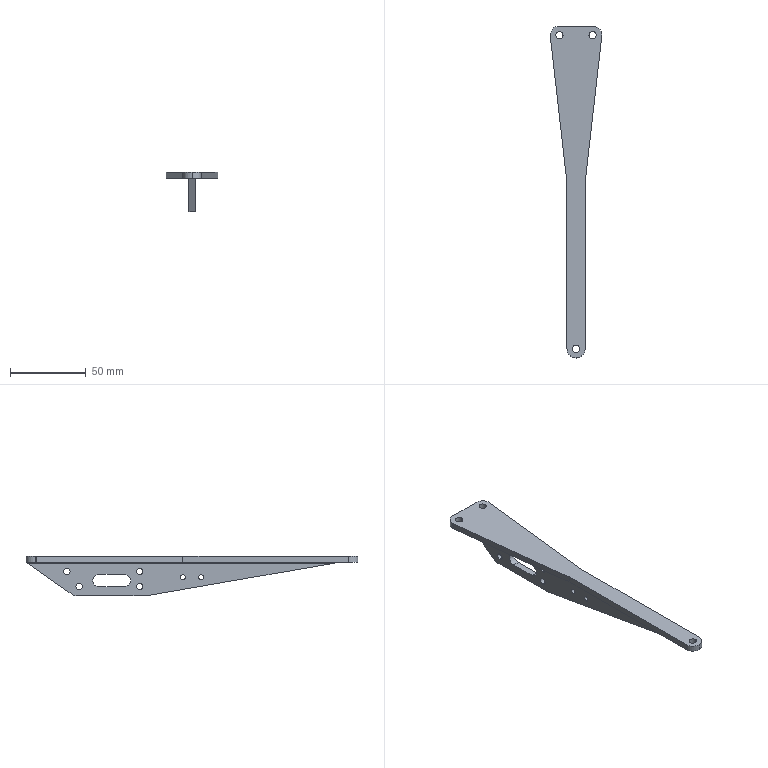Part | SolidWorks | features BaseBody 1 | 1 solid | 44 faces | box 34 x 219 x 26 mm | volume 25249 mm3 | cylinder 29 | plane 15 | commonest cylinder face diameters 4.2 x8 4.9 x6 12 x5 3.2 x4 2 x2 8 x2
STEP:
#1=CARTESIAN_POINT('',(2.,103.5,-12.2));
#2=VERTEX_POINT('',#1);
#3=CARTESIAN_POINT('',(2.,103.5,-15.4));
#4=VERTEX_POINT('',#3);
#5=CARTESIAN_POINT('',(2.,103.5,-13.8));
#6=DIRECTION('',(1.,0.,0.));
#7=DIRECTION('',(0.,0.,1.));
#8=AXIS2_PLACEMENT_3D('',#5,#6,#7);
#9=CIRCLE('',#8,1.6);
#10=EDGE_CURVE('',#2,#4,#9,.T.);
#11=ORIENTED_EDGE('',*,*,#10,.T.);
#12=CARTESIAN_POINT('',(-2.,103.5,-15.4));
#13=VERTEX_POINT('',#12);
#14=CARTESIAN_POINT('',(2.,103.5,-15.4));
#15=DIRECTION('',(-1.,0.,0.));
#16=VECTOR('',#15,1000.);
#17=LINE('',#14,#16);
#18=EDGE_CURVE('',#4,#13,#17,.T.);
#19=ORIENTED_EDGE('',*,*,#18,.T.);
#20=CARTESIAN_POINT('',(-2.,103.5,-12.2));
#21=VERTEX_POINT('',#20);
#22=CARTESIAN_POINT('',(-2.,103.5,-13.8));
#23=DIRECTION('',(-1.,0.,0.));
#24=DIRECTION('',(0.,0.,1.));
#25=AXIS2_PLACEMENT_3D('',#22,#23,#24);
#26=CIRCLE('',#25,1.6);
#27=EDGE_CURVE('',#13,#21,#26,.T.);
#28=ORIENTED_EDGE('',*,*,#27,.T.);
#29=CARTESIAN_POINT('',(2.,103.5,-12.2));
#30=DIRECTION('',(-1.,0.,0.));
#31=VECTOR('',#30,1000.);
#32=LINE('',#29,#31);
#33=EDGE_CURVE('',#2,#21,#32,.T.);
#34=ORIENTED_EDGE('',*,*,#33,.F.);
#35=EDGE_LOOP('',(#11,#19,#28,#34));
#36=FACE_OUTER_BOUND('',#35,.T.);
#37=CARTESIAN_POINT('',(2.,103.5,-13.8));
#38=DIRECTION('',(-1.,0.,0.));
#39=DIRECTION('',(0.,0.,1.));
#40=AXIS2_PLACEMENT_3D('',#37,#38,#39);
#41=CYLINDRICAL_SURFACE('',#40,1.6);
#42=ADVANCED_FACE('',(#36),#41,.F.);
#43=CARTESIAN_POINT('',(2.,184.,-17.9));
#44=VERTEX_POINT('',#43);
#45=CARTESIAN_POINT('',(2.,184.,-22.1));
#46=VERTEX_POINT('',#45);
#47=CARTESIAN_POINT('',(2.,184.,-20.));
#48=DIRECTION('',(1.,0.,0.));
#49=DIRECTION('',(0.,0.,1.));
#50=AXIS2_PLACEMENT_3D('',#47,#48,#49);
#51=CIRCLE('',#50,2.1);
#52=EDGE_CURVE('',#44,#46,#51,.T.);
#53=ORIENTED_EDGE('',*,*,#52,.T.);
#54=CARTESIAN_POINT('',(-2.,184.,-22.1));
#55=VERTEX_POINT('',#54);
#56=CARTESIAN_POINT('',(2.,184.,-22.1));
#57=DIRECTION('',(-1.,0.,0.));
#58=VECTOR('',#57,1000.);
#59=LINE('',#56,#58);
#60=EDGE_CURVE('',#46,#55,#59,.T.);
#61=ORIENTED_EDGE('',*,*,#60,.T.);
#62=CARTESIAN_POINT('',(-2.,184.,-17.9));
#63=VERTEX_POINT('',#62);
#64=CARTESIAN_POINT('',(-2.,184.,-20.));
#65=DIRECTION('',(-1.,0.,0.));
#66=DIRECTION('',(0.,0.,1.));
#67=AXIS2_PLACEMENT_3D('',#64,#65,#66);
#68=CIRCLE('',#67,2.1);
#69=EDGE_CURVE('',#55,#63,#68,.T.);
#70=ORIENTED_EDGE('',*,*,#69,.T.);
#71=CARTESIAN_POINT('',(2.,184.,-17.9));
#72=DIRECTION('',(-1.,0.,0.));
#73=VECTOR('',#72,1000.);
#74=LINE('',#71,#73);
#75=EDGE_CURVE('',#44,#63,#74,.T.);
#76=ORIENTED_EDGE('',*,*,#75,.F.);
#77=EDGE_LOOP('',(#53,#61,#70,#76));
#78=FACE_OUTER_BOUND('',#77,.T.);
#79=CARTESIAN_POINT('',(2.,184.,-20.));
#80=DIRECTION('',(-1.,0.,0.));
#81=DIRECTION('',(0.,0.,1.));
#82=AXIS2_PLACEMENT_3D('',#79,#80,#81);
#83=CYLINDRICAL_SURFACE('',#82,2.1);
#84=ADVANCED_FACE('',(#78),#83,.F.);
#85=CARTESIAN_POINT('',(2.,192.,-7.9));
#86=VERTEX_POINT('',#85);
#87=CARTESIAN_POINT('',(2.,192.,-12.1));
#88=VERTEX_POINT('',#87);
#89=CARTESIAN_POINT('',(2.,192.,-10.));
#90=DIRECTION('',(1.,0.,0.));
#91=DIRECTION('',(0.,0.,1.));
#92=AXIS2_PLACEMENT_3D('',#89,#90,#91);
#93=CIRCLE('',#92,2.1);
#94=EDGE_CURVE('',#86,#88,#93,.T.);
#95=ORIENTED_EDGE('',*,*,#94,.T.);
#96=CARTESIAN_POINT('',(-2.,192.,-12.1));
#97=VERTEX_POINT('',#96);
#98=CARTESIAN_POINT('',(2.,192.,-12.1));
#99=DIRECTION('',(-1.,0.,0.));
#100=VECTOR('',#99,1000.);
#101=LINE('',#98,#100);
#102=EDGE_CURVE('',#88,#97,#101,.T.);
#103=ORIENTED_EDGE('',*,*,#102,.T.);
#104=CARTESIAN_POINT('',(-2.,192.,-7.9));
#105=VERTEX_POINT('',#104);
#106=CARTESIAN_POINT('',(-2.,192.,-10.));
#107=DIRECTION('',(-1.,0.,0.));
#108=DIRECTION('',(0.,0.,1.));
#109=AXIS2_PLACEMENT_3D('',#106,#107,#108);
#110=CIRCLE('',#109,2.1);
#111=EDGE_CURVE('',#97,#105,#110,.T.);
#112=ORIENTED_EDGE('',*,*,#111,.T.);
#113=CARTESIAN_POINT('',(2.,192.,-7.9));
#114=DIRECTION('',(-1.,0.,0.));
#115=VECTOR('',#114,1000.);
#116=LINE('',#113,#115);
#117=EDGE_CURVE('',#86,#105,#116,.T.);
#118=ORIENTED_EDGE('',*,*,#117,.F.);
#119=EDGE_LOOP('',(#95,#103,#112,#118));
#120=FACE_OUTER_BOUND('',#119,.T.);
#121=CARTESIAN_POINT('',(2.,192.,-10.));
#122=DIRECTION('',(-1.,0.,0.));
#123=DIRECTION('',(0.,0.,1.));
#124=AXIS2_PLACEMENT_3D('',#121,#122,#123);
#125=CYLINDRICAL_SURFACE('',#124,2.1);
#126=ADVANCED_FACE('',(#120),#125,.F.);
#127=CARTESIAN_POINT('',(2.,144.,-17.9));
#128=VERTEX_POINT('',#127);
#129=CARTESIAN_POINT('',(2.,144.,-22.1));
#130=VERTEX_POINT('',#129);
#131=CARTESIAN_POINT('',(2.,144.,-20.));
#132=DIRECTION('',(1.,0.,0.));
#133=DIRECTION('',(0.,0.,1.));
#134=AXIS2_PLACEMENT_3D('',#131,#132,#133);
#135=CIRCLE('',#134,2.1);
#136=EDGE_CURVE('',#128,#130,#135,.T.);
#137=ORIENTED_EDGE('',*,*,#136,.T.);
#138=CARTESIAN_POINT('',(-2.,144.,-22.1));
#139=VERTEX_POINT('',#138);
#140=CARTESIAN_POINT('',(2.,144.,-22.1));
#141=DIRECTION('',(-1.,0.,0.));
#142=VECTOR('',#141,1000.);
#143=LINE('',#140,#142);
#144=EDGE_CURVE('',#130,#139,#143,.T.);
#145=ORIENTED_EDGE('',*,*,#144,.T.);
#146=CARTESIAN_POINT('',(-2.,144.,-17.9));
#147=VERTEX_POINT('',#146);
#148=CARTESIAN_POINT('',(-2.,144.,-20.));
#149=DIRECTION('',(-1.,0.,0.));
#150=DIRECTION('',(0.,0.,1.));
#151=AXIS2_PLACEMENT_3D('',#148,#149,#150);
#152=CIRCLE('',#151,2.1);
#153=EDGE_CURVE('',#139,#147,#152,.T.);
#154=ORIENTED_EDGE('',*,*,#153,.T.);
#155=CARTESIAN_POINT('',(2.,144.,-17.9));
#156=DIRECTION('',(-1.,0.,0.));
#157=VECTOR('',#156,1000.);
#158=LINE('',#155,#157);
#159=EDGE_CURVE('',#128,#147,#158,.T.);
#160=ORIENTED_EDGE('',*,*,#159,.F.);
#161=EDGE_LOOP('',(#137,#145,#154,#160));
#162=FACE_OUTER_BOUND('',#161,.T.);
#163=CARTESIAN_POINT('',(2.,144.,-20.));
#164=DIRECTION('',(-1.,0.,0.));
#165=DIRECTION('',(0.,0.,1.));
#166=AXIS2_PLACEMENT_3D('',#163,#164,#165);
#167=CYLINDRICAL_SURFACE('',#166,2.1);
#168=ADVANCED_FACE('',(#162),#167,.F.);
#169=CARTESIAN_POINT('',(2.,144.,-7.9));
#170=VERTEX_POINT('',#169);
#171=CARTESIAN_POINT('',(2.,144.,-12.1));
#172=VERTEX_POINT('',#171);
#173=CARTESIAN_POINT('',(2.,144.,-10.));
#174=DIRECTION('',(1.,0.,0.));
#175=DIRECTION('',(0.,0.,1.));
#176=AXIS2_PLACEMENT_3D('',#173,#174,#175);
#177=CIRCLE('',#176,2.1);
#178=EDGE_CURVE('',#170,#172,#177,.T.);
#179=ORIENTED_EDGE('',*,*,#178,.T.);
#180=CARTESIAN_POINT('',(-2.,144.,-12.1));
#181=VERTEX_POINT('',#180);
#182=CARTESIAN_POINT('',(2.,144.,-12.1));
#183=DIRECTION('',(-1.,0.,0.));
#184=VECTOR('',#183,1000.);
#185=LINE('',#182,#184);
#186=EDGE_CURVE('',#172,#181,#185,.T.);
#187=ORIENTED_EDGE('',*,*,#186,.T.);
#188=CARTESIAN_POINT('',(-2.,144.,-7.9));
#189=VERTEX_POINT('',#188);
#190=CARTESIAN_POINT('',(-2.,144.,-10.));
#191=DIRECTION('',(-1.,0.,0.));
#192=DIRECTION('',(0.,0.,1.));
#193=AXIS2_PLACEMENT_3D('',#190,#191,#192);
#194=CIRCLE('',#193,2.1);
#195=EDGE_CURVE('',#181,#189,#194,.T.);
#196=ORIENTED_EDGE('',*,*,#195,.T.);
#197=CARTESIAN_POINT('',(2.,144.,-7.9));
#198=DIRECTION('',(-1.,0.,0.));
#199=VECTOR('',#198,1000.);
#200=LINE('',#197,#199);
#201=EDGE_CURVE('',#170,#189,#200,.T.);
#202=ORIENTED_EDGE('',*,*,#201,.F.);
#203=EDGE_LOOP('',(#179,#187,#196,#202));
#204=FACE_OUTER_BOUND('',#203,.T.);
#205=CARTESIAN_POINT('',(2.,144.,-10.));
#206=DIRECTION('',(-1.,0.,0.));
#207=DIRECTION('',(0.,0.,1.));
#208=AXIS2_PLACEMENT_3D('',#205,#206,#207);
#209=CYLINDRICAL_SURFACE('',#208,2.1);
#210=ADVANCED_FACE('',(#204),#209,.F.);
#211=CARTESIAN_POINT('',(2.,115.5,-12.2));
#212=VERTEX_POINT('',#211);
#213=CARTESIAN_POINT('',(2.,115.5,-15.4));
#214=VERTEX_POINT('',#213);
#215=CARTESIAN_POINT('',(2.,115.5,-13.8));
#216=DIRECTION('',(1.,0.,0.));
#217=DIRECTION('',(0.,0.,1.));
#218=AXIS2_PLACEMENT_3D('',#215,#216,#217);
#219=CIRCLE('',#218,1.6);
#220=EDGE_CURVE('',#212,#214,#219,.T.);
#221=ORIENTED_EDGE('',*,*,#220,.T.);
#222=CARTESIAN_POINT('',(-2.,115.5,-15.4));
#223=VERTEX_POINT('',#222);
#224=CARTESIAN_POINT('',(2.,115.5,-15.4));
#225=DIRECTION('',(-1.,0.,0.));
#226=VECTOR('',#225,1000.);
#227=LINE('',#224,#226);
#228=EDGE_CURVE('',#214,#223,#227,.T.);
#229=ORIENTED_EDGE('',*,*,#228,.T.);
#230=CARTESIAN_POINT('',(-2.,115.5,-12.2));
#231=VERTEX_POINT('',#230);
#232=CARTESIAN_POINT('',(-2.,115.5,-13.8));
#233=DIRECTION('',(-1.,0.,0.));
#234=DIRECTION('',(0.,0.,1.));
#235=AXIS2_PLACEMENT_3D('',#232,#233,#234);
#236=CIRCLE('',#235,1.6);
#237=EDGE_CURVE('',#223,#231,#236,.T.);
#238=ORIENTED_EDGE('',*,*,#237,.T.);
#239=CARTESIAN_POINT('',(2.,115.5,-12.2));
#240=DIRECTION('',(-1.,0.,0.));
#241=VECTOR('',#240,1000.);
#242=LINE('',#239,#241);
#243=EDGE_CURVE('',#212,#231,#242,.T.);
#244=ORIENTED_EDGE('',*,*,#243,.F.);
#245=EDGE_LOOP('',(#221,#229,#238,#244));
#246=FACE_OUTER_BOUND('',#245,.T.);
#247=CARTESIAN_POINT('',(2.,115.5,-13.8));
#248=DIRECTION('',(-1.,0.,0.));
#249=DIRECTION('',(0.,0.,1.));
#250=AXIS2_PLACEMENT_3D('',#247,#248,#249);
#251=CYLINDRICAL_SURFACE('',#250,1.6);
#252=ADVANCED_FACE('',(#246),#251,.F.);
#253=CARTESIAN_POINT('',(8.55,213.,0.));
#254=VERTEX_POINT('',#253);
#255=CARTESIAN_POINT('',(13.45,213.,0.));
#256=VERTEX_POINT('',#255);
#257=CARTESIAN_POINT('',(11.,213.,0.));
#258=DIRECTION('',(0.,0.,1.));
#259=DIRECTION('',(-1.,0.,0.));
#260=AXIS2_PLACEMENT_3D('',#257,#258,#259);
#261=CIRCLE('',#260,2.45);
#262=EDGE_CURVE('',#254,#256,#261,.T.);
#263=ORIENTED_EDGE('',*,*,#262,.T.);
#264=CARTESIAN_POINT('',(13.45,213.,-4.));
#265=VERTEX_POINT('',#264);
#266=CARTESIAN_POINT('',(13.45,213.,0.));
#267=DIRECTION('',(0.,0.,-1.));
#268=VECTOR('',#267,1000.);
#269=LINE('',#266,#268);
#270=EDGE_CURVE('',#256,#265,#269,.T.);
#271=ORIENTED_EDGE('',*,*,#270,.T.);
#272=CARTESIAN_POINT('',(8.55,213.,-4.));
#273=VERTEX_POINT('',#272);
#274=CARTESIAN_POINT('',(11.,213.,-4.));
#275=DIRECTION('',(0.,0.,-1.));
#276=DIRECTION('',(-1.,0.,0.));
#277=AXIS2_PLACEMENT_3D('',#274,#275,#276);
#278=CIRCLE('',#277,2.45);
#279=EDGE_CURVE('',#265,#273,#278,.T.);
#280=ORIENTED_EDGE('',*,*,#279,.T.);
#281=CARTESIAN_POINT('',(8.55,213.,0.));
#282=DIRECTION('',(0.,0.,-1.));
#283=VECTOR('',#282,1000.);
#284=LINE('',#281,#283);
#285=EDGE_CURVE('',#254,#273,#284,.T.);
#286=ORIENTED_EDGE('',*,*,#285,.F.);
#287=EDGE_LOOP('',(#263,#271,#280,#286));
#288=FACE_OUTER_BOUND('',#287,.T.);
#289=CARTESIAN_POINT('',(11.,213.,0.));
#290=DIRECTION('',(0.,0.,-1.));
#291=DIRECTION('',(-1.,0.,0.));
#292=AXIS2_PLACEMENT_3D('',#289,#290,#291);
#293=CYLINDRICAL_SURFACE('',#292,2.45);
#294=ADVANCED_FACE('',(#288),#293,.F.);
#295=CARTESIAN_POINT('',(-2.45,6.,0.));
#296=VERTEX_POINT('',#295);
#297=CARTESIAN_POINT('',(2.45,6.,0.));
#298=VERTEX_POINT('',#297);
#299=CARTESIAN_POINT('',(0.,6.,0.));
#300=DIRECTION('',(0.,0.,1.));
#301=DIRECTION('',(-1.,0.,0.));
#302=AXIS2_PLACEMENT_3D('',#299,#300,#301);
#303=CIRCLE('',#302,2.45);
#304=EDGE_CURVE('',#296,#298,#303,.T.);
#305=ORIENTED_EDGE('',*,*,#304,.T.);
#306=CARTESIAN_POINT('',(2.45,6.,-4.));
#307=VERTEX_POINT('',#306);
#308=CARTESIAN_POINT('',(2.45,6.,0.));
#309=DIRECTION('',(0.,0.,-1.));
#310=VECTOR('',#309,1000.);
#311=LINE('',#308,#310);
#312=EDGE_CURVE('',#298,#307,#311,.T.);
#313=ORIENTED_EDGE('',*,*,#312,.T.);
#314=CARTESIAN_POINT('',(-2.45,6.,-4.));
#315=VERTEX_POINT('',#314);
#316=CARTESIAN_POINT('',(0.,6.,-4.));
#317=DIRECTION('',(0.,0.,-1.));
#318=DIRECTION('',(-1.,0.,0.));
#319=AXIS2_PLACEMENT_3D('',#316,#317,#318);
#320=CIRCLE('',#319,2.45);
#321=EDGE_CURVE('',#307,#315,#320,.T.);
#322=ORIENTED_EDGE('',*,*,#321,.T.);
#323=CARTESIAN_POINT('',(-2.45,6.,0.));
#324=DIRECTION('',(0.,0.,-1.));
#325=VECTOR('',#324,1000.);
#326=LINE('',#323,#325);
#327=EDGE_CURVE('',#296,#315,#326,.T.);
#328=ORIENTED_EDGE('',*,*,#327,.F.);
#329=EDGE_LOOP('',(#305,#313,#322,#328));
#330=FACE_OUTER_BOUND('',#329,.T.);
#331=CARTESIAN_POINT('',(0.,6.,0.));
#332=DIRECTION('',(0.,0.,-1.));
#333=DIRECTION('',(-1.,0.,0.));
#334=AXIS2_PLACEMENT_3D('',#331,#332,#333);
#335=CYLINDRICAL_SURFACE('',#334,2.45);
#336=ADVANCED_FACE('',(#330),#335,.F.);
#337=CARTESIAN_POINT('',(-13.45,213.,0.));
#338=VERTEX_POINT('',#337);
#339=CARTESIAN_POINT('',(-8.55,213.,0.));
#340=VERTEX_POINT('',#339);
#341=CARTESIAN_POINT('',(-11.,213.,0.));
#342=DIRECTION('',(0.,0.,1.));
#343=DIRECTION('',(-1.,0.,0.));
#344=AXIS2_PLACEMENT_3D('',#341,#342,#343);
#345=CIRCLE('',#344,2.45);
#346=EDGE_CURVE('',#338,#340,#345,.T.);
#347=ORIENTED_EDGE('',*,*,#346,.T.);
#348=CARTESIAN_POINT('',(-8.55,213.,-4.));
#349=VERTEX_POINT('',#348);
#350=CARTESIAN_POINT('',(-8.55,213.,0.));
#351=DIRECTION('',(0.,0.,-1.));
#352=VECTOR('',#351,1000.);
#353=LINE('',#350,#352);
#354=EDGE_CURVE('',#340,#349,#353,.T.);
#355=ORIENTED_EDGE('',*,*,#354,.T.);
#356=CARTESIAN_POINT('',(-13.45,213.,-4.));
#357=VERTEX_POINT('',#356);
#358=CARTESIAN_POINT('',(-11.,213.,-4.));
#359=DIRECTION('',(0.,0.,-1.));
#360=DIRECTION('',(-1.,0.,0.));
#361=AXIS2_PLACEMENT_3D('',#358,#359,#360);
#362=CIRCLE('',#361,2.45);
#363=EDGE_CURVE('',#349,#357,#362,.T.);
#364=ORIENTED_EDGE('',*,*,#363,.T.);
#365=CARTESIAN_POINT('',(-13.45,213.,0.));
#366=DIRECTION('',(0.,0.,-1.));
#367=VECTOR('',#366,1000.);
#368=LINE('',#365,#367);
#369=EDGE_CURVE('',#338,#357,#368,.T.);
#370=ORIENTED_EDGE('',*,*,#369,.F.);
#371=EDGE_LOOP('',(#347,#355,#364,#370));
#372=FACE_OUTER_BOUND('',#371,.T.);
#373=CARTESIAN_POINT('',(-11.,213.,0.));
#374=DIRECTION('',(0.,0.,-1.));
#375=DIRECTION('',(-1.,0.,0.));
#376=AXIS2_PLACEMENT_3D('',#373,#374,#375);
#377=CYLINDRICAL_SURFACE('',#376,2.45);
#378=ADVANCED_FACE('',(#372),#377,.F.);
#379=CARTESIAN_POINT('',(-17.,213.,0.));
#380=VERTEX_POINT('',#379);
#381=CARTESIAN_POINT('',(-16.962,212.325,0.));
#382=VERTEX_POINT('',#381);
#383=CARTESIAN_POINT('',(-11.,213.,0.));
#384=DIRECTION('',(0.,0.,1.));
#385=DIRECTION('',(-1.,0.,0.));
#386=AXIS2_PLACEMENT_3D('',#383,#384,#385);
#387=CIRCLE('',#386,6.);
#388=EDGE_CURVE('',#380,#382,#387,.T.);
#389=ORIENTED_EDGE('',*,*,#388,.F.);
#390=CARTESIAN_POINT('',(-17.,213.,-4.));
#391=VERTEX_POINT('',#390);
#392=CARTESIAN_POINT('',(-17.,213.,0.));
#393=DIRECTION('',(0.,0.,-1.));
#394=VECTOR('',#393,1000.);
#395=LINE('',#392,#394);
#396=EDGE_CURVE('',#380,#391,#395,.T.);
#397=ORIENTED_EDGE('',*,*,#396,.T.);
#398=CARTESIAN_POINT('',(-16.962,212.325,-4.));
#399=VERTEX_POINT('',#398);
#400=CARTESIAN_POINT('',(-11.,213.,-4.));
#401=DIRECTION('',(0.,0.,1.));
#402=DIRECTION('',(-1.,0.,0.));
#403=AXIS2_PLACEMENT_3D('',#400,#401,#402);
#404=CIRCLE('',#403,6.);
#405=EDGE_CURVE('',#391,#399,#404,.T.);
#406=ORIENTED_EDGE('',*,*,#405,.T.);
#407=CARTESIAN_POINT('',(-16.962,212.325,-2.));
#408=DIRECTION('',(0.,0.,-1.));
#409=VECTOR('',#408,1000.);
#410=LINE('',#407,#409);
#411=EDGE_CURVE('',#382,#399,#410,.T.);
#412=ORIENTED_EDGE('',*,*,#411,.F.);
#413=EDGE_LOOP('',(#389,#397,#406,#412));
#414=FACE_OUTER_BOUND('',#413,.T.);
#415=CARTESIAN_POINT('',(-11.,213.,0.));
#416=DIRECTION('',(0.,0.,-1.));
#417=DIRECTION('',(-1.,0.,0.));
#418=AXIS2_PLACEMENT_3D('',#415,#416,#417);
#419=CYLINDRICAL_SURFACE('',#418,6.);
#420=ADVANCED_FACE('',(#414),#419,.T.);
#421=ORIENTED_EDGE('',*,*,#18,.F.);
#422=CARTESIAN_POINT('',(2.,103.5,-13.8));
#423=DIRECTION('',(1.,0.,0.));
#424=DIRECTION('',(0.,0.,1.));
#425=AXIS2_PLACEMENT_3D('',#422,#423,#424);
#426=CIRCLE('',#425,1.6);
#427=EDGE_CURVE('',#4,#2,#426,.T.);
#428=ORIENTED_EDGE('',*,*,#427,.T.);
#429=ORIENTED_EDGE('',*,*,#33,.T.);
#430=CARTESIAN_POINT('',(-2.,103.5,-13.8));
#431=DIRECTION('',(-1.,0.,0.));
#432=DIRECTION('',(0.,0.,1.));
#433=AXIS2_PLACEMENT_3D('',#430,#431,#432);
#434=CIRCLE('',#433,1.6);
#435=EDGE_CURVE('',#21,#13,#434,.T.);
#436=ORIENTED_EDGE('',*,*,#435,.T.);
#437=EDGE_LOOP('',(#421,#428,#429,#436));
#438=FACE_OUTER_BOUND('',#437,.T.);
#439=CARTESIAN_POINT('',(2.,103.5,-13.8));
#440=DIRECTION('',(-1.,0.,0.));
#441=DIRECTION('',(0.,0.,1.));
#442=AXIS2_PLACEMENT_3D('',#439,#440,#441);
#443=CYLINDRICAL_SURFACE('',#442,1.6);
#444=ADVANCED_FACE('',(#438),#443,.F.);
#445=CARTESIAN_POINT('',(-2.,184.,-20.));
#446=DIRECTION('',(-1.,0.,0.));
#447=DIRECTION('',(0.,0.,1.));
#448=AXIS2_PLACEMENT_3D('',#445,#446,#447);
#449=CIRCLE('',#448,2.1);
#450=EDGE_CURVE('',#63,#55,#449,.T.);
#451=ORIENTED_EDGE('',*,*,#450,.F.);
#452=ORIENTED_EDGE('',*,*,#69,.F.);
#453=EDGE_LOOP('',(#451,#452));
#454=FACE_BOUND('',#453,.T.);
#455=CARTESIAN_POINT('',(-2.,192.,-10.));
#456=DIRECTION('',(-1.,0.,0.));
#457=DIRECTION('',(0.,0.,1.));
#458=AXIS2_PLACEMENT_3D('',#455,#456,#457);
#459=CIRCLE('',#458,2.1);
#460=EDGE_CURVE('',#105,#97,#459,.T.);
#461=ORIENTED_EDGE('',*,*,#460,.F.);
#462=ORIENTED_EDGE('',*,*,#111,.F.);
#463=EDGE_LOOP('',(#461,#462));
#464=FACE_BOUND('',#463,.T.);
#465=CARTESIAN_POINT('',(-2.,144.,-20.));
#466=DIRECTION('',(-1.,0.,0.));
#467=DIRECTION('',(0.,0.,1.));
#468=AXIS2_PLACEMENT_3D('',#465,#466,#467);
#469=CIRCLE('',#468,2.1);
#470=EDGE_CURVE('',#147,#139,#469,.T.);
#471=ORIENTED_EDGE('',*,*,#470,.F.);
#472=ORIENTED_EDGE('',*,*,#153,.F.);
#473=EDGE_LOOP('',(#471,#472));
#474=FACE_BOUND('',#473,.T.);
#475=CARTESIAN_POINT('',(-2.,144.,-10.));
#476=DIRECTION('',(-1.,0.,0.));
#477=DIRECTION('',(0.,0.,1.));
#478=AXIS2_PLACEMENT_3D('',#475,#476,#477);
#479=CIRCLE('',#478,2.1);
#480=EDGE_CURVE('',#189,#181,#479,.T.);
#481=ORIENTED_EDGE('',*,*,#480,.F.);
#482=ORIENTED_EDGE('',*,*,#195,.F.);
#483=EDGE_LOOP('',(#481,#482));
#484=FACE_BOUND('',#483,.T.);
#485=CARTESIAN_POINT('',(-2.,115.5,-13.8));
#486=DIRECTION('',(-1.,0.,0.));
#487=DIRECTION('',(0.,0.,1.));
#488=AXIS2_PLACEMENT_3D('',#485,#486,#487);
#489=CIRCLE('',#488,1.6);
#490=EDGE_CURVE('',#231,#223,#489,.T.);
#491=ORIENTED_EDGE('',*,*,#490,.F.);
#492=ORIENTED_EDGE('',*,*,#237,.F.);
#493=EDGE_LOOP('',(#491,#492));
#494=FACE_BOUND('',#493,.T.);
#495=CARTESIAN_POINT('',(-2.,171.,-12.));
#496=VERTEX_POINT('',#495);
#497=CARTESIAN_POINT('',(-2.,171.,-20.));
#498=VERTEX_POINT('',#497);
#499=CARTESIAN_POINT('',(-2.,171.,-16.));
#500=DIRECTION('',(-1.,0.,0.));
#501=DIRECTION('',(0.,0.,1.));
#502=AXIS2_PLACEMENT_3D('',#499,#500,#501);
#503=CIRCLE('',#502,4.);
#504=EDGE_CURVE('',#496,#498,#503,.T.);
#505=ORIENTED_EDGE('',*,*,#504,.F.);
#506=CARTESIAN_POINT('',(-2.,154.,-12.));
#507=VERTEX_POINT('',#506);
#508=CARTESIAN_POINT('',(-2.,117.919,-12.));
#509=DIRECTION('',(0.,1.,0.));
#510=VECTOR('',#509,1000.);
#511=LINE('',#508,#510);
#512=EDGE_CURVE('',#507,#496,#511,.T.);
#513=ORIENTED_EDGE('',*,*,#512,.F.);
#514=CARTESIAN_POINT('',(-2.,154.,-20.));
#515=VERTEX_POINT('',#514);
#516=CARTESIAN_POINT('',(-2.,154.,-16.));
#517=DIRECTION('',(-1.,0.,0.));
#518=DIRECTION('',(0.,0.,1.));
#519=AXIS2_PLACEMENT_3D('',#516,#517,#518);
#520=CIRCLE('',#519,4.);
#521=EDGE_CURVE('',#515,#507,#520,.T.);
#522=ORIENTED_EDGE('',*,*,#521,.F.);
#523=CARTESIAN_POINT('',(-2.,117.919,-20.));
#524=DIRECTION('',(0.,-1.,0.));
#525=VECTOR('',#524,1000.);
#526=LINE('',#523,#525);
#527=EDGE_CURVE('',#498,#515,#526,.T.);
#528=ORIENTED_EDGE('',*,*,#527,.F.);
#529=EDGE_LOOP('',(#505,#513,#522,#528));
#530=FACE_BOUND('',#529,.T.);
#531=ORIENTED_EDGE('',*,*,#435,.F.);
#532=ORIENTED_EDGE('',*,*,#27,.F.);
#533=EDGE_LOOP('',(#531,#532));
#534=FACE_BOUND('',#533,.T.);
#535=CARTESIAN_POINT('',(-2.,139.751,-26.));
#536=VERTEX_POINT('',#535);
#537=CARTESIAN_POINT('',(-2.,138.897,-25.926));
#538=VERTEX_POINT('',#537);
#539=CARTESIAN_POINT('',(-2.,139.751,-21.));
#540=DIRECTION('',(-1.,0.,0.));
#541=DIRECTION('',(0.,0.,1.));
#542=AXIS2_PLACEMENT_3D('',#539,#540,#541);
#543=CIRCLE('',#542,5.);
#544=EDGE_CURVE('',#536,#538,#543,.T.);
#545=ORIENTED_EDGE('',*,*,#544,.T.);
#546=CARTESIAN_POINT('',(-2.,18.277,-5.));
#547=VERTEX_POINT('',#546);
#548=CARTESIAN_POINT('',(-2.,138.897,-25.926));
#549=DIRECTION('',(0.,0.9853,-0.1709));
#550=VECTOR('',#549,1000.);
#551=LINE('',#548,#550);
#552=EDGE_CURVE('',#547,#538,#551,.T.);
#553=ORIENTED_EDGE('',*,*,#552,.F.);
#554=CARTESIAN_POINT('',(-2.,217.561,-5.));
#555=VERTEX_POINT('',#554);
#556=CARTESIAN_POINT('',(-2.,117.919,-5.));
#557=DIRECTION('',(0.,-1.,0.));
#558=VECTOR('',#557,1000.);
#559=LINE('',#556,#558);
#560=EDGE_CURVE('',#555,#547,#559,.T.);
#561=ORIENTED_EDGE('',*,*,#560,.F.);
#562=CARTESIAN_POINT('',(-2.,188.626,-25.106));
#563=VERTEX_POINT('',#562);
#564=CARTESIAN_POINT('',(-2.,219.,-4.));
#565=DIRECTION('',(0.,0.8212,0.5706));
#566=VECTOR('',#565,1000.);
#567=LINE('',#564,#566);
#568=EDGE_CURVE('',#563,#555,#567,.T.);
#569=ORIENTED_EDGE('',*,*,#568,.F.);
#570=CARTESIAN_POINT('',(-2.,185.773,-26.));
#571=VERTEX_POINT('',#570);
#572=CARTESIAN_POINT('',(-2.,185.773,-21.));
#573=DIRECTION('',(1.,0.,0.));
#574=DIRECTION('',(0.,0.,1.));
#575=AXIS2_PLACEMENT_3D('',#572,#573,#574);
#576=CIRCLE('',#575,5.);
#577=EDGE_CURVE('',#571,#563,#576,.T.);
#578=ORIENTED_EDGE('',*,*,#577,.F.);
#579=CARTESIAN_POINT('',(-2.,117.919,-26.));
#580=DIRECTION('',(0.,1.,0.));
#581=VECTOR('',#580,1000.);
#582=LINE('',#579,#581);
#583=EDGE_CURVE('',#536,#571,#582,.T.);
#584=ORIENTED_EDGE('',*,*,#583,.F.);
#585=EDGE_LOOP('',(#545,#553,#561,#569,#578,#584));
#586=FACE_OUTER_BOUND('',#585,.T.);
#587=CARTESIAN_POINT('',(-2.,17.081,-5.));
#588=DIRECTION('',(1.,0.,0.));
#589=DIRECTION('',(0.,0.,-1.));
#590=AXIS2_PLACEMENT_3D('',#587,#588,#589);
#591=PLANE('',#590);
#592=ADVANCED_FACE('',(#454,#464,#474,#484,#494,#530,#534,#586),#591,.F.);
#593=ORIENTED_EDGE('',*,*,#52,.F.);
#594=CARTESIAN_POINT('',(2.,184.,-20.));
#595=DIRECTION('',(1.,0.,0.));
#596=DIRECTION('',(0.,0.,1.));
#597=AXIS2_PLACEMENT_3D('',#594,#595,#596);
#598=CIRCLE('',#597,2.1);
#599=EDGE_CURVE('',#46,#44,#598,.T.);
#600=ORIENTED_EDGE('',*,*,#599,.F.);
#601=EDGE_LOOP('',(#593,#600));
#602=FACE_BOUND('',#601,.T.);
#603=ORIENTED_EDGE('',*,*,#94,.F.);
#604=CARTESIAN_POINT('',(2.,192.,-10.));
#605=DIRECTION('',(1.,0.,0.));
#606=DIRECTION('',(0.,0.,1.));
#607=AXIS2_PLACEMENT_3D('',#604,#605,#606);
#608=CIRCLE('',#607,2.1);
#609=EDGE_CURVE('',#88,#86,#608,.T.);
#610=ORIENTED_EDGE('',*,*,#609,.F.);
#611=EDGE_LOOP('',(#603,#610));
#612=FACE_BOUND('',#611,.T.);
#613=ORIENTED_EDGE('',*,*,#136,.F.);
#614=CARTESIAN_POINT('',(2.,144.,-20.));
#615=DIRECTION('',(1.,0.,0.));
#616=DIRECTION('',(0.,0.,1.));
#617=AXIS2_PLACEMENT_3D('',#614,#615,#616);
#618=CIRCLE('',#617,2.1);
#619=EDGE_CURVE('',#130,#128,#618,.T.);
#620=ORIENTED_EDGE('',*,*,#619,.F.);
#621=EDGE_LOOP('',(#613,#620));
#622=FACE_BOUND('',#621,.T.);
#623=ORIENTED_EDGE('',*,*,#178,.F.);
#624=CARTESIAN_POINT('',(2.,144.,-10.));
#625=DIRECTION('',(1.,0.,0.));
#626=DIRECTION('',(0.,0.,1.));
#627=AXIS2_PLACEMENT_3D('',#624,#625,#626);
#628=CIRCLE('',#627,2.1);
#629=EDGE_CURVE('',#172,#170,#628,.T.);
#630=ORIENTED_EDGE('',*,*,#629,.F.);
#631=EDGE_LOOP('',(#623,#630));
#632=FACE_BOUND('',#631,.T.);
#633=ORIENTED_EDGE('',*,*,#220,.F.);
#634=CARTESIAN_POINT('',(2.,115.5,-13.8));
#635=DIRECTION('',(1.,0.,0.));
#636=DIRECTION('',(0.,0.,1.));
#637=AXIS2_PLACEMENT_3D('',#634,#635,#636);
#638=CIRCLE('',#637,1.6);
#639=EDGE_CURVE('',#214,#212,#638,.T.);
#640=ORIENTED_EDGE('',*,*,#639,.F.);
#641=EDGE_LOOP('',(#633,#640));
#642=FACE_BOUND('',#641,.T.);
#643=CARTESIAN_POINT('',(2.,171.,-20.));
#644=VERTEX_POINT('',#643);
#645=CARTESIAN_POINT('',(2.,171.,-12.));
#646=VERTEX_POINT('',#645);
#647=CARTESIAN_POINT('',(2.,171.,-16.));
#648=DIRECTION('',(1.,0.,0.));
#649=DIRECTION('',(0.,0.,1.));
#650=AXIS2_PLACEMENT_3D('',#647,#648,#649);
#651=CIRCLE('',#650,4.);
#652=EDGE_CURVE('',#644,#646,#651,.T.);
#653=ORIENTED_EDGE('',*,*,#652,.F.);
#654=CARTESIAN_POINT('',(2.,154.,-20.));
#655=VERTEX_POINT('',#654);
#656=CARTESIAN_POINT('',(2.,117.919,-20.));
#657=DIRECTION('',(0.,1.,0.));
#658=VECTOR('',#657,1000.);
#659=LINE('',#656,#658);
#660=EDGE_CURVE('',#655,#644,#659,.T.);
#661=ORIENTED_EDGE('',*,*,#660,.F.);
#662=CARTESIAN_POINT('',(2.,154.,-12.));
#663=VERTEX_POINT('',#662);
#664=CARTESIAN_POINT('',(2.,154.,-16.));
#665=DIRECTION('',(1.,0.,0.));
#666=DIRECTION('',(0.,0.,1.));
#667=AXIS2_PLACEMENT_3D('',#664,#665,#666);
#668=CIRCLE('',#667,4.);
#669=EDGE_CURVE('',#663,#655,#668,.T.);
#670=ORIENTED_EDGE('',*,*,#669,.F.);
#671=CARTESIAN_POINT('',(2.,117.919,-12.));
#672=DIRECTION('',(0.,-1.,0.));
#673=VECTOR('',#672,1000.);
#674=LINE('',#671,#673);
#675=EDGE_CURVE('',#646,#663,#674,.T.);
#676=ORIENTED_EDGE('',*,*,#675,.F.);
#677=EDGE_LOOP('',(#653,#661,#670,#676));
#678=FACE_BOUND('',#677,.T.);
#679=ORIENTED_EDGE('',*,*,#10,.F.);
#680=ORIENTED_EDGE('',*,*,#427,.F.);
#681=EDGE_LOOP('',(#679,#680));
#682=FACE_BOUND('',#681,.T.);
#683=CARTESIAN_POINT('',(2.,138.897,-25.926));
#684=VERTEX_POINT('',#683);
#685=CARTESIAN_POINT('',(2.,139.751,-26.));
#686=VERTEX_POINT('',#685);
#687=CARTESIAN_POINT('',(2.,139.751,-21.));
#688=DIRECTION('',(1.,0.,0.));
#689=DIRECTION('',(0.,0.,1.));
#690=AXIS2_PLACEMENT_3D('',#687,#688,#689);
#691=CIRCLE('',#690,5.);
#692=EDGE_CURVE('',#684,#686,#691,.T.);
#693=ORIENTED_EDGE('',*,*,#692,.T.);
#694=CARTESIAN_POINT('',(2.,185.773,-26.));
#695=VERTEX_POINT('',#694);
#696=CARTESIAN_POINT('',(2.,117.919,-26.));
#697=DIRECTION('',(0.,-1.,0.));
#698=VECTOR('',#697,1000.);
#699=LINE('',#696,#698);
#700=EDGE_CURVE('',#695,#686,#699,.T.);
#701=ORIENTED_EDGE('',*,*,#700,.F.);
#702=CARTESIAN_POINT('',(2.,188.626,-25.106));
#703=VERTEX_POINT('',#702);
#704=CARTESIAN_POINT('',(2.,185.773,-21.));
#705=DIRECTION('',(-1.,0.,0.));
#706=DIRECTION('',(0.,0.,1.));
#707=AXIS2_PLACEMENT_3D('',#704,#705,#706);
#708=CIRCLE('',#707,5.);
#709=EDGE_CURVE('',#703,#695,#708,.T.);
#710=ORIENTED_EDGE('',*,*,#709,.F.);
#711=CARTESIAN_POINT('',(2.,217.561,-5.));
#712=VERTEX_POINT('',#711);
#713=CARTESIAN_POINT('',(2.,219.,-4.));
#714=DIRECTION('',(0.,-0.8212,-0.5706));
#715=VECTOR('',#714,1000.);
#716=LINE('',#713,#715);
#717=EDGE_CURVE('',#712,#703,#716,.T.);
#718=ORIENTED_EDGE('',*,*,#717,.F.);
#719=CARTESIAN_POINT('',(2.,18.277,-5.));
#720=VERTEX_POINT('',#719);
#721=CARTESIAN_POINT('',(2.,117.919,-5.));
#722=DIRECTION('',(0.,1.,0.));
#723=VECTOR('',#722,1000.);
#724=LINE('',#721,#723);
#725=EDGE_CURVE('',#720,#712,#724,.T.);
#726=ORIENTED_EDGE('',*,*,#725,.F.);
#727=CARTESIAN_POINT('',(2.,138.897,-25.926));
#728=DIRECTION('',(0.,-0.9853,0.1709));
#729=VECTOR('',#728,1000.);
#730=LINE('',#727,#729);
#731=EDGE_CURVE('',#684,#720,#730,.T.);
#732=ORIENTED_EDGE('',*,*,#731,.F.);
#733=EDGE_LOOP('',(#693,#701,#710,#718,#726,#732));
#734=FACE_OUTER_BOUND('',#733,.T.);
#735=CARTESIAN_POINT('',(2.,17.081,-26.));
#736=DIRECTION('',(-1.,0.,0.));
#737=DIRECTION('',(0.,0.,1.));
#738=AXIS2_PLACEMENT_3D('',#735,#736,#737);
#739=PLANE('',#738);
#740=ADVANCED_FACE('',(#602,#612,#622,#632,#642,#678,#682,#734),#739,.F.);
#741=ORIENTED_EDGE('',*,*,#60,.F.);
#742=ORIENTED_EDGE('',*,*,#599,.T.);
#743=ORIENTED_EDGE('',*,*,#75,.T.);
#744=ORIENTED_EDGE('',*,*,#450,.T.);
#745=EDGE_LOOP('',(#741,#742,#743,#744));
#746=FACE_OUTER_BOUND('',#745,.T.);
#747=CARTESIAN_POINT('',(2.,184.,-20.));
#748=DIRECTION('',(-1.,0.,0.));
#749=DIRECTION('',(0.,0.,1.));
#750=AXIS2_PLACEMENT_3D('',#747,#748,#749);
#751=CYLINDRICAL_SURFACE('',#750,2.1);
#752=ADVANCED_FACE('',(#746),#751,.F.);
#753=ORIENTED_EDGE('',*,*,#102,.F.);
#754=ORIENTED_EDGE('',*,*,#609,.T.);
#755=ORIENTED_EDGE('',*,*,#117,.T.);
#756=ORIENTED_EDGE('',*,*,#460,.T.);
#757=EDGE_LOOP('',(#753,#754,#755,#756));
#758=FACE_OUTER_BOUND('',#757,.T.);
#759=CARTESIAN_POINT('',(2.,192.,-10.));
#760=DIRECTION('',(-1.,0.,0.));
#761=DIRECTION('',(0.,0.,1.));
#762=AXIS2_PLACEMENT_3D('',#759,#760,#761);
#763=CYLINDRICAL_SURFACE('',#762,2.1);
#764=ADVANCED_FACE('',(#758),#763,.F.);
#765=ORIENTED_EDGE('',*,*,#144,.F.);
#766=ORIENTED_EDGE('',*,*,#619,.T.);
#767=ORIENTED_EDGE('',*,*,#159,.T.);
#768=ORIENTED_EDGE('',*,*,#470,.T.);
#769=EDGE_LOOP('',(#765,#766,#767,#768));
#770=FACE_OUTER_BOUND('',#769,.T.);
#771=CARTESIAN_POINT('',(2.,144.,-20.));
#772=DIRECTION('',(-1.,0.,0.));
#773=DIRECTION('',(0.,0.,1.));
#774=AXIS2_PLACEMENT_3D('',#771,#772,#773);
#775=CYLINDRICAL_SURFACE('',#774,2.1);
#776=ADVANCED_FACE('',(#770),#775,.F.);
#777=ORIENTED_EDGE('',*,*,#186,.F.);
#778=ORIENTED_EDGE('',*,*,#629,.T.);
#779=ORIENTED_EDGE('',*,*,#201,.T.);
#780=ORIENTED_EDGE('',*,*,#480,.T.);
#781=EDGE_LOOP('',(#777,#778,#779,#780));
#782=FACE_OUTER_BOUND('',#781,.T.);
#783=CARTESIAN_POINT('',(2.,144.,-10.));
#784=DIRECTION('',(-1.,0.,0.));
#785=DIRECTION('',(0.,0.,1.));
#786=AXIS2_PLACEMENT_3D('',#783,#784,#785);
#787=CYLINDRICAL_SURFACE('',#786,2.1);
#788=ADVANCED_FACE('',(#782),#787,.F.);
#789=ORIENTED_EDGE('',*,*,#228,.F.);
#790=ORIENTED_EDGE('',*,*,#639,.T.);
#791=ORIENTED_EDGE('',*,*,#243,.T.);
#792=ORIENTED_EDGE('',*,*,#490,.T.);
#793=EDGE_LOOP('',(#789,#790,#791,#792));
#794=FACE_OUTER_BOUND('',#793,.T.);
#795=CARTESIAN_POINT('',(2.,115.5,-13.8));
#796=DIRECTION('',(-1.,0.,0.));
#797=DIRECTION('',(0.,0.,1.));
#798=AXIS2_PLACEMENT_3D('',#795,#796,#797);
#799=CYLINDRICAL_SURFACE('',#798,1.6);
#800=ADVANCED_FACE('',(#794),#799,.F.);
#801=ORIENTED_EDGE('',*,*,#527,.T.);
#802=CARTESIAN_POINT('',(0.,154.,-20.));
#803=DIRECTION('',(-1.,0.,0.));
#804=VECTOR('',#803,1000.);
#805=LINE('',#802,#804);
#806=EDGE_CURVE('',#655,#515,#805,.T.);
#807=ORIENTED_EDGE('',*,*,#806,.F.);
#808=ORIENTED_EDGE('',*,*,#660,.T.);
#809=CARTESIAN_POINT('',(0.,171.,-20.));
#810=DIRECTION('',(1.,0.,0.));
#811=VECTOR('',#810,1000.);
#812=LINE('',#809,#811);
#813=EDGE_CURVE('',#498,#644,#812,.T.);
#814=ORIENTED_EDGE('',*,*,#813,.F.);
#815=EDGE_LOOP('',(#801,#807,#808,#814));
#816=FACE_OUTER_BOUND('',#815,.T.);
#817=CARTESIAN_POINT('',(-2.,154.,-20.));
#818=DIRECTION('',(0.,0.,-1.));
#819=DIRECTION('',(0.,1.,0.));
#820=AXIS2_PLACEMENT_3D('',#817,#818,#819);
#821=PLANE('',#820);
#822=ADVANCED_FACE('',(#816),#821,.F.);
#823=ORIENTED_EDGE('',*,*,#813,.T.);
#824=ORIENTED_EDGE('',*,*,#652,.T.);
#825=CARTESIAN_POINT('',(0.,171.,-12.));
#826=DIRECTION('',(-1.,0.,0.));
#827=VECTOR('',#826,1000.);
#828=LINE('',#825,#827);
#829=EDGE_CURVE('',#646,#496,#828,.T.);
#830=ORIENTED_EDGE('',*,*,#829,.T.);
#831=ORIENTED_EDGE('',*,*,#504,.T.);
#832=EDGE_LOOP('',(#823,#824,#830,#831));
#833=FACE_OUTER_BOUND('',#832,.T.);
#834=CARTESIAN_POINT('',(2.,171.,-16.));
#835=DIRECTION('',(-1.,0.,0.));
#836=DIRECTION('',(0.,0.,1.));
#837=AXIS2_PLACEMENT_3D('',#834,#835,#836);
#838=CYLINDRICAL_SURFACE('',#837,4.);
#839=ADVANCED_FACE('',(#833),#838,.F.);
#840=ORIENTED_EDGE('',*,*,#512,.T.);
#841=ORIENTED_EDGE('',*,*,#829,.F.);
#842=ORIENTED_EDGE('',*,*,#675,.T.);
#843=CARTESIAN_POINT('',(0.,154.,-12.));
#844=DIRECTION('',(1.,0.,0.));
#845=VECTOR('',#844,1000.);
#846=LINE('',#843,#845);
#847=EDGE_CURVE('',#507,#663,#846,.T.);
#848=ORIENTED_EDGE('',*,*,#847,.F.);
#849=EDGE_LOOP('',(#840,#841,#842,#848));
#850=FACE_OUTER_BOUND('',#849,.T.);
#851=CARTESIAN_POINT('',(-2.,171.,-12.));
#852=DIRECTION('',(0.,0.,1.));
#853=DIRECTION('',(0.,-1.,0.));
#854=AXIS2_PLACEMENT_3D('',#851,#852,#853);
#855=PLANE('',#854);
#856=ADVANCED_FACE('',(#850),#855,.F.);
#857=ORIENTED_EDGE('',*,*,#847,.T.);
#858=ORIENTED_EDGE('',*,*,#669,.T.);
#859=ORIENTED_EDGE('',*,*,#806,.T.);
#860=ORIENTED_EDGE('',*,*,#521,.T.);
#861=EDGE_LOOP('',(#857,#858,#859,#860));
#862=FACE_OUTER_BOUND('',#861,.T.);
#863=CARTESIAN_POINT('',(2.,154.,-16.));
#864=DIRECTION('',(-1.,0.,0.));
#865=DIRECTION('',(0.,0.,1.));
#866=AXIS2_PLACEMENT_3D('',#863,#864,#865);
#867=CYLINDRICAL_SURFACE('',#866,4.);
#868=ADVANCED_FACE('',(#862),#867,.F.);
#869=CARTESIAN_POINT('',(0.,139.751,-26.));
#870=DIRECTION('',(1.,0.,0.));
#871=VECTOR('',#870,1000.);
#872=LINE('',#869,#871);
#873=EDGE_CURVE('',#536,#686,#872,.T.);
#874=ORIENTED_EDGE('',*,*,#873,.F.);
#875=ORIENTED_EDGE('',*,*,#583,.T.);
#876=CARTESIAN_POINT('',(0.,185.773,-26.));
#877=DIRECTION('',(-1.,0.,0.));
#878=VECTOR('',#877,1000.);
#879=LINE('',#876,#878);
#880=EDGE_CURVE('',#695,#571,#879,.T.);
#881=ORIENTED_EDGE('',*,*,#880,.F.);
#882=ORIENTED_EDGE('',*,*,#700,.T.);
#883=EDGE_LOOP('',(#874,#875,#881,#882));
#884=FACE_OUTER_BOUND('',#883,.T.);
#885=CARTESIAN_POINT('',(-2.,139.751,-26.));
#886=DIRECTION('',(0.,0.,1.));
#887=DIRECTION('',(1.,0.,0.));
#888=AXIS2_PLACEMENT_3D('',#885,#886,#887);
#889=PLANE('',#888);
#890=ADVANCED_FACE('',(#884),#889,.F.);
#891=CARTESIAN_POINT('',(0.,138.897,-25.926));
#892=DIRECTION('',(-1.,0.,0.));
#893=VECTOR('',#892,1000.);
#894=LINE('',#891,#893);
#895=EDGE_CURVE('',#684,#538,#894,.T.);
#896=ORIENTED_EDGE('',*,*,#895,.F.);
#897=ORIENTED_EDGE('',*,*,#731,.T.);
#898=CARTESIAN_POINT('',(3.,12.513,-4.));
#899=VERTEX_POINT('',#898);
#900=CARTESIAN_POINT('',(3.,12.513,-4.));
#901=CARTESIAN_POINT('',(2.414,12.513,-4.));
#902=CARTESIAN_POINT('',(2.,14.901,-4.414));
#903=CARTESIAN_POINT('',(2.,18.277,-5.));
#904=(BOUNDED_CURVE()B_SPLINE_CURVE(3,(#900,#901,#902,#903),.UNSPECIFIED.,.F.,.F.)B_SPLINE_CURVE_WITH_KNOTS((4,4),(0.,1.571),.UNSPECIFIED.)CURVE()GEOMETRIC_REPRESENTATION_ITEM()RATIONAL_B_SPLINE_CURVE((1.,0.8047,0.8047,1.))REPRESENTATION_ITEM(''));
#905=EDGE_CURVE('',#899,#720,#904,.T.);
#906=ORIENTED_EDGE('',*,*,#905,.F.);
#907=CARTESIAN_POINT('',(-3.,12.513,-4.));
#908=VERTEX_POINT('',#907);
#909=CARTESIAN_POINT('',(0.,12.513,-4.));
#910=DIRECTION('',(1.,0.,0.));
#911=VECTOR('',#910,1000.);
#912=LINE('',#909,#911);
#913=EDGE_CURVE('',#908,#899,#912,.T.);
#914=ORIENTED_EDGE('',*,*,#913,.F.);
#915=CARTESIAN_POINT('',(-2.,18.277,-5.));
#916=CARTESIAN_POINT('',(-2.,14.901,-4.414));
#917=CARTESIAN_POINT('',(-2.414,12.513,-4.));
#918=CARTESIAN_POINT('',(-3.,12.513,-4.));
#919=(BOUNDED_CURVE()B_SPLINE_CURVE(3,(#915,#916,#917,#918),.UNSPECIFIED.,.F.,.F.)B_SPLINE_CURVE_WITH_KNOTS((4,4),(4.712,6.283),.UNSPECIFIED.)CURVE()GEOMETRIC_REPRESENTATION_ITEM()RATIONAL_B_SPLINE_CURVE((1.,0.8047,0.8047,1.))REPRESENTATION_ITEM(''));
#920=EDGE_CURVE('',#547,#908,#919,.T.);
#921=ORIENTED_EDGE('',*,*,#920,.F.);
#922=ORIENTED_EDGE('',*,*,#552,.T.);
#923=EDGE_LOOP('',(#896,#897,#906,#914,#921,#922));
#924=FACE_OUTER_BOUND('',#923,.T.);
#925=CARTESIAN_POINT('',(-3.036,138.897,-25.926));
#926=DIRECTION('',(0.,0.1709,0.9853));
#927=DIRECTION('',(0.,-0.9853,0.1709));
#928=AXIS2_PLACEMENT_3D('',#925,#926,#927);
#929=PLANE('',#928);
#930=ADVANCED_FACE('',(#924),#929,.F.);
#931=ORIENTED_EDGE('',*,*,#560,.T.);
#932=ORIENTED_EDGE('',*,*,#920,.T.);
#933=CARTESIAN_POINT('',(-3.,219.,-4.));
#934=VERTEX_POINT('',#933);
#935=CARTESIAN_POINT('',(-3.,115.756,-4.));
#936=DIRECTION('',(0.,1.,0.));
#937=VECTOR('',#936,1000.);
#938=LINE('',#935,#937);
#939=EDGE_CURVE('',#908,#934,#938,.T.);
#940=ORIENTED_EDGE('',*,*,#939,.T.);
#941=CARTESIAN_POINT('',(-3.,219.,-4.));
#942=CARTESIAN_POINT('',(-2.414,219.,-4.));
#943=CARTESIAN_POINT('',(-2.,218.404,-4.414));
#944=CARTESIAN_POINT('',(-2.,217.561,-5.));
#945=(BOUNDED_CURVE()B_SPLINE_CURVE(3,(#941,#942,#943,#944),.UNSPECIFIED.,.F.,.T.)B_SPLINE_CURVE_WITH_KNOTS((4,4),(3.142,4.712),.UNSPECIFIED.)CURVE()GEOMETRIC_REPRESENTATION_ITEM()RATIONAL_B_SPLINE_CURVE((1.,0.8047,0.8047,1.))REPRESENTATION_ITEM(''));
#946=EDGE_CURVE('',#934,#555,#945,.T.);
#947=ORIENTED_EDGE('',*,*,#946,.T.);
#948=EDGE_LOOP('',(#931,#932,#940,#947));
#949=FACE_OUTER_BOUND('',#948,.T.);
#950=CARTESIAN_POINT('',(-3.,220.239,-5.));
#951=DIRECTION('',(0.,-1.,0.));
#952=DIRECTION('',(0.,0.,-1.));
#953=AXIS2_PLACEMENT_3D('',#950,#951,#952);
#954=CYLINDRICAL_SURFACE('',#953,1.);
#955=ADVANCED_FACE('',(#949),#954,.F.);
#956=CARTESIAN_POINT('',(0.,188.626,-25.106));
#957=DIRECTION('',(1.,0.,0.));
#958=VECTOR('',#957,1000.);
#959=LINE('',#956,#958);
#960=EDGE_CURVE('',#563,#703,#959,.T.);
#961=ORIENTED_EDGE('',*,*,#960,.F.);
#962=ORIENTED_EDGE('',*,*,#568,.T.);
#963=ORIENTED_EDGE('',*,*,#946,.F.);
#964=CARTESIAN_POINT('',(3.,219.,-4.));
#965=VERTEX_POINT('',#964);
#966=CARTESIAN_POINT('',(0.,219.,-4.));
#967=DIRECTION('',(-1.,0.,0.));
#968=VECTOR('',#967,1000.);
#969=LINE('',#966,#968);
#970=EDGE_CURVE('',#965,#934,#969,.T.);
#971=ORIENTED_EDGE('',*,*,#970,.F.);
#972=CARTESIAN_POINT('',(2.,217.561,-5.));
#973=CARTESIAN_POINT('',(2.,218.404,-4.414));
#974=CARTESIAN_POINT('',(2.414,219.,-4.));
#975=CARTESIAN_POINT('',(3.,219.,-4.));
#976=(BOUNDED_CURVE()B_SPLINE_CURVE(3,(#972,#973,#974,#975),.UNSPECIFIED.,.F.,.F.)B_SPLINE_CURVE_WITH_KNOTS((4,4),(1.571,3.142),.UNSPECIFIED.)CURVE()GEOMETRIC_REPRESENTATION_ITEM()RATIONAL_B_SPLINE_CURVE((1.,0.8047,0.8047,1.))REPRESENTATION_ITEM(''));
#977=EDGE_CURVE('',#712,#965,#976,.T.);
#978=ORIENTED_EDGE('',*,*,#977,.F.);
#979=ORIENTED_EDGE('',*,*,#717,.T.);
#980=EDGE_LOOP('',(#961,#962,#963,#971,#978,#979));
#981=FACE_OUTER_BOUND('',#980,.T.);
#982=CARTESIAN_POINT('',(-3.036,219.,-4.));
#983=DIRECTION('',(0.,-0.5706,0.8212));
#984=DIRECTION('',(0.,-0.8212,-0.5706));
#985=AXIS2_PLACEMENT_3D('',#982,#983,#984);
#986=PLANE('',#985);
#987=ADVANCED_FACE('',(#981),#986,.F.);
#988=ORIENTED_EDGE('',*,*,#880,.T.);
#989=ORIENTED_EDGE('',*,*,#577,.T.);
#990=ORIENTED_EDGE('',*,*,#960,.T.);
#991=ORIENTED_EDGE('',*,*,#709,.T.);
#992=EDGE_LOOP('',(#988,#989,#990,#991));
#993=FACE_OUTER_BOUND('',#992,.T.);
#994=CARTESIAN_POINT('',(2.,185.773,-21.));
#995=DIRECTION('',(-1.,0.,0.));
#996=DIRECTION('',(0.,0.,1.));
#997=AXIS2_PLACEMENT_3D('',#994,#995,#996);
#998=CYLINDRICAL_SURFACE('',#997,5.);
#999=ADVANCED_FACE('',(#993),#998,.T.);
#1000=CARTESIAN_POINT('',(3.,115.756,-4.));
#1001=DIRECTION('',(0.,-1.,0.));
#1002=VECTOR('',#1001,1000.);
#1003=LINE('',#1000,#1002);
#1004=EDGE_CURVE('',#965,#899,#1003,.T.);
#1005=ORIENTED_EDGE('',*,*,#1004,.T.);
#1006=ORIENTED_EDGE('',*,*,#905,.T.);
#1007=ORIENTED_EDGE('',*,*,#725,.T.);
#1008=ORIENTED_EDGE('',*,*,#977,.T.);
#1009=EDGE_LOOP('',(#1005,#1006,#1007,#1008));
#1010=FACE_OUTER_BOUND('',#1009,.T.);
#1011=CARTESIAN_POINT('',(3.,220.239,-5.));
#1012=DIRECTION('',(0.,-1.,0.));
#1013=DIRECTION('',(0.,0.,-1.));
#1014=AXIS2_PLACEMENT_3D('',#1011,#1012,#1013);
#1015=CYLINDRICAL_SURFACE('',#1014,1.);
#1016=ADVANCED_FACE('',(#1010),#1015,.F.);
#1017=ORIENTED_EDGE('',*,*,#895,.T.);
#1018=ORIENTED_EDGE('',*,*,#544,.F.);
#1019=ORIENTED_EDGE('',*,*,#873,.T.);
#1020=ORIENTED_EDGE('',*,*,#692,.F.);
#1021=EDGE_LOOP('',(#1017,#1018,#1019,#1020));
#1022=FACE_OUTER_BOUND('',#1021,.T.);
#1023=CARTESIAN_POINT('',(2.,139.751,-21.));
#1024=DIRECTION('',(-1.,0.,0.));
#1025=DIRECTION('',(0.,0.,1.));
#1026=AXIS2_PLACEMENT_3D('',#1023,#1024,#1025);
#1027=CYLINDRICAL_SURFACE('',#1026,5.);
#1028=ADVANCED_FACE('',(#1022),#1027,.T.);
#1029=CARTESIAN_POINT('',(11.,213.,-4.));
#1030=DIRECTION('',(0.,0.,-1.));
#1031=DIRECTION('',(-1.,0.,0.));
#1032=AXIS2_PLACEMENT_3D('',#1029,#1030,#1031);
#1033=CIRCLE('',#1032,2.45);
#1034=EDGE_CURVE('',#273,#265,#1033,.T.);
#1035=ORIENTED_EDGE('',*,*,#1034,.F.);
#1036=ORIENTED_EDGE('',*,*,#279,.F.);
#1037=EDGE_LOOP('',(#1035,#1036));
#1038=FACE_BOUND('',#1037,.T.);
#1039=CARTESIAN_POINT('',(0.,6.,-4.));
#1040=DIRECTION('',(0.,0.,-1.));
#1041=DIRECTION('',(-1.,0.,0.));
#1042=AXIS2_PLACEMENT_3D('',#1039,#1040,#1041);
#1043=CIRCLE('',#1042,2.45);
#1044=EDGE_CURVE('',#315,#307,#1043,.T.);
#1045=ORIENTED_EDGE('',*,*,#1044,.F.);
#1046=ORIENTED_EDGE('',*,*,#321,.F.);
#1047=EDGE_LOOP('',(#1045,#1046));
#1048=FACE_BOUND('',#1047,.T.);
#1049=CARTESIAN_POINT('',(-11.,213.,-4.));
#1050=DIRECTION('',(0.,0.,-1.));
#1051=DIRECTION('',(-1.,0.,0.));
#1052=AXIS2_PLACEMENT_3D('',#1049,#1050,#1051);
#1053=CIRCLE('',#1052,2.45);
#1054=EDGE_CURVE('',#357,#349,#1053,.T.);
#1055=ORIENTED_EDGE('',*,*,#1054,.F.);
#1056=ORIENTED_EDGE('',*,*,#363,.F.);
#1057=EDGE_LOOP('',(#1055,#1056));
#1058=FACE_BOUND('',#1057,.T.);
#1059=ORIENTED_EDGE('',*,*,#913,.T.);
#1060=ORIENTED_EDGE('',*,*,#1004,.F.);
#1061=CARTESIAN_POINT('',(11.,219.,-4.));
#1062=VERTEX_POINT('',#1061);
#1063=CARTESIAN_POINT('',(0.,219.,-4.));
#1064=DIRECTION('',(-1.,0.,0.));
#1065=VECTOR('',#1064,1000.);
#1066=LINE('',#1063,#1065);
#1067=EDGE_CURVE('',#1062,#965,#1066,.T.);
#1068=ORIENTED_EDGE('',*,*,#1067,.F.);
#1069=CARTESIAN_POINT('',(16.962,212.325,-4.));
#1070=VERTEX_POINT('',#1069);
#1071=CARTESIAN_POINT('',(11.,213.,-4.));
#1072=DIRECTION('',(0.,0.,1.));
#1073=DIRECTION('',(-1.,0.,0.));
#1074=AXIS2_PLACEMENT_3D('',#1071,#1072,#1073);
#1075=CIRCLE('',#1074,6.);
#1076=EDGE_CURVE('',#1070,#1062,#1075,.T.);
#1077=ORIENTED_EDGE('',*,*,#1076,.F.);
#1078=CARTESIAN_POINT('',(6.,115.5,-4.));
#1079=VERTEX_POINT('',#1078);
#1080=CARTESIAN_POINT('',(16.962,212.325,-4.));
#1081=DIRECTION('',(0.1125,0.9937,0.));
#1082=VECTOR('',#1081,1000.);
#1083=LINE('',#1080,#1082);
#1084=EDGE_CURVE('',#1079,#1070,#1083,.T.);
#1085=ORIENTED_EDGE('',*,*,#1084,.F.);
#1086=CARTESIAN_POINT('',(6.,6.,-4.));
#1087=VERTEX_POINT('',#1086);
#1088=CARTESIAN_POINT('',(6.,109.5,-4.));
#1089=DIRECTION('',(0.,1.,0.));
#1090=VECTOR('',#1089,1000.);
#1091=LINE('',#1088,#1090);
#1092=EDGE_CURVE('',#1087,#1079,#1091,.T.);
#1093=ORIENTED_EDGE('',*,*,#1092,.F.);
#1094=CARTESIAN_POINT('',(0.01869,0.,-4.));
#1095=VERTEX_POINT('',#1094);
#1096=CARTESIAN_POINT('',(0.,6.,-4.));
#1097=DIRECTION('',(0.,0.,1.));
#1098=DIRECTION('',(-1.,0.,0.));
#1099=AXIS2_PLACEMENT_3D('',#1096,#1097,#1098);
#1100=CIRCLE('',#1099,6.);
#1101=EDGE_CURVE('',#1095,#1087,#1100,.T.);
#1102=ORIENTED_EDGE('',*,*,#1101,.F.);
#1103=CARTESIAN_POINT('',(-0.01869,0.,-4.));
#1104=VERTEX_POINT('',#1103);
#1105=CARTESIAN_POINT('',(0.,0.,-4.));
#1106=DIRECTION('',(-1.,0.,0.));
#1107=VECTOR('',#1106,1000.);
#1108=LINE('',#1105,#1107);
#1109=EDGE_CURVE('',#1095,#1104,#1108,.T.);
#1110=ORIENTED_EDGE('',*,*,#1109,.T.);
#1111=CARTESIAN_POINT('',(-6.,6.,-4.));
#1112=VERTEX_POINT('',#1111);
#1113=CARTESIAN_POINT('',(0.,6.,-4.));
#1114=DIRECTION('',(0.,0.,1.));
#1115=DIRECTION('',(-1.,0.,0.));
#1116=AXIS2_PLACEMENT_3D('',#1113,#1114,#1115);
#1117=CIRCLE('',#1116,6.);
#1118=EDGE_CURVE('',#1112,#1104,#1117,.T.);
#1119=ORIENTED_EDGE('',*,*,#1118,.F.);
#1120=CARTESIAN_POINT('',(-6.,115.5,-4.));
#1121=VERTEX_POINT('',#1120);
#1122=CARTESIAN_POINT('',(-6.,109.5,-4.));
#1123=DIRECTION('',(0.,-1.,0.));
#1124=VECTOR('',#1123,1000.);
#1125=LINE('',#1122,#1124);
#1126=EDGE_CURVE('',#1121,#1112,#1125,.T.);
#1127=ORIENTED_EDGE('',*,*,#1126,.F.);
#1128=CARTESIAN_POINT('',(-16.962,212.325,-4.));
#1129=DIRECTION('',(0.1125,-0.9937,0.));
#1130=VECTOR('',#1129,1000.);
#1131=LINE('',#1128,#1130);
#1132=EDGE_CURVE('',#399,#1121,#1131,.T.);
#1133=ORIENTED_EDGE('',*,*,#1132,.F.);
#1134=ORIENTED_EDGE('',*,*,#405,.F.);
#1135=CARTESIAN_POINT('',(-11.,219.,-4.));
#1136=VERTEX_POINT('',#1135);
#1137=CARTESIAN_POINT('',(-11.,213.,-4.));
#1138=DIRECTION('',(0.,0.,1.));
#1139=DIRECTION('',(-1.,0.,0.));
#1140=AXIS2_PLACEMENT_3D('',#1137,#1138,#1139);
#1141=CIRCLE('',#1140,6.);
#1142=EDGE_CURVE('',#1136,#391,#1141,.T.);
#1143=ORIENTED_EDGE('',*,*,#1142,.F.);
#1144=CARTESIAN_POINT('',(0.,219.,-4.));
#1145=DIRECTION('',(-1.,0.,0.));
#1146=VECTOR('',#1145,1000.);
#1147=LINE('',#1144,#1146);
#1148=EDGE_CURVE('',#934,#1136,#1147,.T.);
#1149=ORIENTED_EDGE('',*,*,#1148,.F.);
#1150=ORIENTED_EDGE('',*,*,#939,.F.);
#1151=EDGE_LOOP('',(#1059,#1060,#1068,#1077,#1085,#1093,#1102,#1110,#1119,#1127,#1133,#1134,#1143,#1149,#1150));
#1152=FACE_OUTER_BOUND('',#1151,.T.);
#1153=CARTESIAN_POINT('',(-17.204,0.,-4.));
#1154=DIRECTION('',(0.,0.,1.));
#1155=DIRECTION('',(1.,0.,0.));
#1156=AXIS2_PLACEMENT_3D('',#1153,#1154,#1155);
#1157=PLANE('',#1156);
#1158=ADVANCED_FACE('',(#1038,#1048,#1058,#1152),#1157,.F.);
#1159=CARTESIAN_POINT('',(11.,219.,0.));
#1160=VERTEX_POINT('',#1159);
#1161=CARTESIAN_POINT('',(11.,219.,-2.));
#1162=DIRECTION('',(0.,0.,-1.));
#1163=VECTOR('',#1162,1000.);
#1164=LINE('',#1161,#1163);
#1165=EDGE_CURVE('',#1160,#1062,#1164,.T.);
#1166=ORIENTED_EDGE('',*,*,#1165,.T.);
#1167=ORIENTED_EDGE('',*,*,#1067,.T.);
#1168=ORIENTED_EDGE('',*,*,#970,.T.);
#1169=ORIENTED_EDGE('',*,*,#1148,.T.);
#1170=CARTESIAN_POINT('',(-11.,219.,0.));
#1171=VERTEX_POINT('',#1170);
#1172=CARTESIAN_POINT('',(-11.,219.,-2.));
#1173=DIRECTION('',(0.,0.,1.));
#1174=VECTOR('',#1173,1000.);
#1175=LINE('',#1172,#1174);
#1176=EDGE_CURVE('',#1136,#1171,#1175,.T.);
#1177=ORIENTED_EDGE('',*,*,#1176,.T.);
#1178=CARTESIAN_POINT('',(0.,219.,0.));
#1179=DIRECTION('',(1.,0.,0.));
#1180=VECTOR('',#1179,1000.);
#1181=LINE('',#1178,#1180);
#1182=EDGE_CURVE('',#1171,#1160,#1181,.T.);
#1183=ORIENTED_EDGE('',*,*,#1182,.T.);
#1184=EDGE_LOOP('',(#1166,#1167,#1168,#1169,#1177,#1183));
#1185=FACE_OUTER_BOUND('',#1184,.T.);
#1186=CARTESIAN_POINT('',(-11.,219.,-4.));
#1187=DIRECTION('',(0.,1.,0.));
#1188=DIRECTION('',(0.,0.,1.));
#1189=AXIS2_PLACEMENT_3D('',#1186,#1187,#1188);
#1190=PLANE('',#1189);
#1191=ADVANCED_FACE('',(#1185),#1190,.T.);
#1192=ORIENTED_EDGE('',*,*,#270,.F.);
#1193=CARTESIAN_POINT('',(11.,213.,0.));
#1194=DIRECTION('',(0.,0.,1.));
#1195=DIRECTION('',(-1.,0.,0.));
#1196=AXIS2_PLACEMENT_3D('',#1193,#1194,#1195);
#1197=CIRCLE('',#1196,2.45);
#1198=EDGE_CURVE('',#256,#254,#1197,.T.);
#1199=ORIENTED_EDGE('',*,*,#1198,.T.);
#1200=ORIENTED_EDGE('',*,*,#285,.T.);
#1201=ORIENTED_EDGE('',*,*,#1034,.T.);
#1202=EDGE_LOOP('',(#1192,#1199,#1200,#1201));
#1203=FACE_OUTER_BOUND('',#1202,.T.);
#1204=CARTESIAN_POINT('',(11.,213.,0.));
#1205=DIRECTION('',(0.,0.,-1.));
#1206=DIRECTION('',(-1.,0.,0.));
#1207=AXIS2_PLACEMENT_3D('',#1204,#1205,#1206);
#1208=CYLINDRICAL_SURFACE('',#1207,2.45);
#1209=ADVANCED_FACE('',(#1203),#1208,.F.);
#1210=ORIENTED_EDGE('',*,*,#312,.F.);
#1211=CARTESIAN_POINT('',(0.,6.,0.));
#1212=DIRECTION('',(0.,0.,1.));
#1213=DIRECTION('',(-1.,0.,0.));
#1214=AXIS2_PLACEMENT_3D('',#1211,#1212,#1213);
#1215=CIRCLE('',#1214,2.45);
#1216=EDGE_CURVE('',#298,#296,#1215,.T.);
#1217=ORIENTED_EDGE('',*,*,#1216,.T.);
#1218=ORIENTED_EDGE('',*,*,#327,.T.);
#1219=ORIENTED_EDGE('',*,*,#1044,.T.);
#1220=EDGE_LOOP('',(#1210,#1217,#1218,#1219));
#1221=FACE_OUTER_BOUND('',#1220,.T.);
#1222=CARTESIAN_POINT('',(0.,6.,0.));
#1223=DIRECTION('',(0.,0.,-1.));
#1224=DIRECTION('',(-1.,0.,0.));
#1225=AXIS2_PLACEMENT_3D('',#1222,#1223,#1224);
#1226=CYLINDRICAL_SURFACE('',#1225,2.45);
#1227=ADVANCED_FACE('',(#1221),#1226,.F.);
#1228=ORIENTED_EDGE('',*,*,#354,.F.);
#1229=CARTESIAN_POINT('',(-11.,213.,0.));
#1230=DIRECTION('',(0.,0.,1.));
#1231=DIRECTION('',(-1.,0.,0.));
#1232=AXIS2_PLACEMENT_3D('',#1229,#1230,#1231);
#1233=CIRCLE('',#1232,2.45);
#1234=EDGE_CURVE('',#340,#338,#1233,.T.);
#1235=ORIENTED_EDGE('',*,*,#1234,.T.);
#1236=ORIENTED_EDGE('',*,*,#369,.T.);
#1237=ORIENTED_EDGE('',*,*,#1054,.T.);
#1238=EDGE_LOOP('',(#1228,#1235,#1236,#1237));
#1239=FACE_OUTER_BOUND('',#1238,.T.);
#1240=CARTESIAN_POINT('',(-11.,213.,0.));
#1241=DIRECTION('',(0.,0.,-1.));
#1242=DIRECTION('',(-1.,0.,0.));
#1243=AXIS2_PLACEMENT_3D('',#1240,#1241,#1242);
#1244=CYLINDRICAL_SURFACE('',#1243,2.45);
#1245=ADVANCED_FACE('',(#1239),#1244,.F.);
#1246=CARTESIAN_POINT('',(16.962,212.325,0.));
#1247=VERTEX_POINT('',#1246);
#1248=CARTESIAN_POINT('',(16.962,212.325,-2.));
#1249=DIRECTION('',(0.,0.,1.));
#1250=VECTOR('',#1249,1000.);
#1251=LINE('',#1248,#1250);
#1252=EDGE_CURVE('',#1070,#1247,#1251,.T.);
#1253=ORIENTED_EDGE('',*,*,#1252,.F.);
#1254=ORIENTED_EDGE('',*,*,#1076,.T.);
#1255=ORIENTED_EDGE('',*,*,#1165,.F.);
#1256=CARTESIAN_POINT('',(11.,213.,0.));
#1257=DIRECTION('',(0.,0.,1.));
#1258=DIRECTION('',(-1.,0.,0.));
#1259=AXIS2_PLACEMENT_3D('',#1256,#1257,#1258);
#1260=CIRCLE('',#1259,6.);
#1261=EDGE_CURVE('',#1247,#1160,#1260,.T.);
#1262=ORIENTED_EDGE('',*,*,#1261,.F.);
#1263=EDGE_LOOP('',(#1253,#1254,#1255,#1262));
#1264=FACE_OUTER_BOUND('',#1263,.T.);
#1265=CARTESIAN_POINT('',(11.,213.,0.));
#1266=DIRECTION('',(0.,0.,-1.));
#1267=DIRECTION('',(-1.,0.,0.));
#1268=AXIS2_PLACEMENT_3D('',#1265,#1266,#1267);
#1269=CYLINDRICAL_SURFACE('',#1268,6.);
#1270=ADVANCED_FACE('',(#1264),#1269,.T.);
#1271=ORIENTED_EDGE('',*,*,#1084,.T.);
#1272=ORIENTED_EDGE('',*,*,#1252,.T.);
#1273=CARTESIAN_POINT('',(6.,115.5,0.));
#1274=VERTEX_POINT('',#1273);
#1275=CARTESIAN_POINT('',(11.481,163.913,0.));
#1276=DIRECTION('',(0.1125,0.9937,0.));
#1277=VECTOR('',#1276,1000.);
#1278=LINE('',#1275,#1277);
#1279=EDGE_CURVE('',#1274,#1247,#1278,.T.);
#1280=ORIENTED_EDGE('',*,*,#1279,.F.);
#1281=CARTESIAN_POINT('',(6.,115.5,-2.));
#1282=DIRECTION('',(0.,0.,1.));
#1283=VECTOR('',#1282,1000.);
#1284=LINE('',#1281,#1283);
#1285=EDGE_CURVE('',#1079,#1274,#1284,.T.);
#1286=ORIENTED_EDGE('',*,*,#1285,.F.);
#1287=EDGE_LOOP('',(#1271,#1272,#1280,#1286));
#1288=FACE_OUTER_BOUND('',#1287,.T.);
#1289=CARTESIAN_POINT('',(16.962,212.325,-4.));
#1290=DIRECTION('',(-0.9937,0.1125,0.));
#1291=DIRECTION('',(-0.1125,-0.9937,0.));
#1292=AXIS2_PLACEMENT_3D('',#1289,#1290,#1291);
#1293=PLANE('',#1292);
#1294=ADVANCED_FACE('',(#1288),#1293,.F.);
#1295=ORIENTED_EDGE('',*,*,#1092,.T.);
#1296=ORIENTED_EDGE('',*,*,#1285,.T.);
#1297=CARTESIAN_POINT('',(6.,6.,0.));
#1298=VERTEX_POINT('',#1297);
#1299=CARTESIAN_POINT('',(6.,60.75,0.));
#1300=DIRECTION('',(0.,-1.,0.));
#1301=VECTOR('',#1300,1000.);
#1302=LINE('',#1299,#1301);
#1303=EDGE_CURVE('',#1274,#1298,#1302,.T.);
#1304=ORIENTED_EDGE('',*,*,#1303,.T.);
#1305=CARTESIAN_POINT('',(6.,6.,-2.));
#1306=DIRECTION('',(0.,0.,-1.));
#1307=VECTOR('',#1306,1000.);
#1308=LINE('',#1305,#1307);
#1309=EDGE_CURVE('',#1298,#1087,#1308,.T.);
#1310=ORIENTED_EDGE('',*,*,#1309,.T.);
#1311=EDGE_LOOP('',(#1295,#1296,#1304,#1310));
#1312=FACE_OUTER_BOUND('',#1311,.T.);
#1313=CARTESIAN_POINT('',(6.,6.,0.));
#1314=DIRECTION('',(1.,0.,0.));
#1315=DIRECTION('',(0.,0.,-1.));
#1316=AXIS2_PLACEMENT_3D('',#1313,#1314,#1315);
#1317=PLANE('',#1316);
#1318=ADVANCED_FACE('',(#1312),#1317,.T.);
#1319=ORIENTED_EDGE('',*,*,#1101,.T.);
#1320=ORIENTED_EDGE('',*,*,#1309,.F.);
#1321=CARTESIAN_POINT('',(0.01869,0.,0.));
#1322=VERTEX_POINT('',#1321);
#1323=CARTESIAN_POINT('',(0.,6.,0.));
#1324=DIRECTION('',(0.,0.,1.));
#1325=DIRECTION('',(-1.,0.,0.));
#1326=AXIS2_PLACEMENT_3D('',#1323,#1324,#1325);
#1327=CIRCLE('',#1326,6.);
#1328=EDGE_CURVE('',#1322,#1298,#1327,.T.);
#1329=ORIENTED_EDGE('',*,*,#1328,.F.);
#1330=CARTESIAN_POINT('',(0.01869,0.,-2.));
#1331=DIRECTION('',(0.,0.,1.));
#1332=VECTOR('',#1331,1000.);
#1333=LINE('',#1330,#1332);
#1334=EDGE_CURVE('',#1095,#1322,#1333,.T.);
#1335=ORIENTED_EDGE('',*,*,#1334,.F.);
#1336=EDGE_LOOP('',(#1319,#1320,#1329,#1335));
#1337=FACE_OUTER_BOUND('',#1336,.T.);
#1338=CARTESIAN_POINT('',(0.,6.,0.));
#1339=DIRECTION('',(0.,0.,-1.));
#1340=DIRECTION('',(-1.,0.,0.));
#1341=AXIS2_PLACEMENT_3D('',#1338,#1339,#1340);
#1342=CYLINDRICAL_SURFACE('',#1341,6.);
#1343=ADVANCED_FACE('',(#1337),#1342,.T.);
#1344=CARTESIAN_POINT('',(-0.01869,0.,0.));
#1345=VERTEX_POINT('',#1344);
#1346=CARTESIAN_POINT('',(-0.01869,0.,-2.));
#1347=DIRECTION('',(0.,0.,-1.));
#1348=VECTOR('',#1347,1000.);
#1349=LINE('',#1346,#1348);
#1350=EDGE_CURVE('',#1345,#1104,#1349,.T.);
#1351=ORIENTED_EDGE('',*,*,#1350,.F.);
#1352=CARTESIAN_POINT('',(-6.,6.,0.));
#1353=VERTEX_POINT('',#1352);
#1354=CARTESIAN_POINT('',(0.,6.,0.));
#1355=DIRECTION('',(0.,0.,1.));
#1356=DIRECTION('',(-1.,0.,0.));
#1357=AXIS2_PLACEMENT_3D('',#1354,#1355,#1356);
#1358=CIRCLE('',#1357,6.);
#1359=EDGE_CURVE('',#1353,#1345,#1358,.T.);
#1360=ORIENTED_EDGE('',*,*,#1359,.F.);
#1361=CARTESIAN_POINT('',(-6.,6.,-2.));
#1362=DIRECTION('',(0.,0.,1.));
#1363=VECTOR('',#1362,1000.);
#1364=LINE('',#1361,#1363);
#1365=EDGE_CURVE('',#1112,#1353,#1364,.T.);
#1366=ORIENTED_EDGE('',*,*,#1365,.F.);
#1367=ORIENTED_EDGE('',*,*,#1118,.T.);
#1368=EDGE_LOOP('',(#1351,#1360,#1366,#1367));
#1369=FACE_OUTER_BOUND('',#1368,.T.);
#1370=CARTESIAN_POINT('',(0.,6.,0.));
#1371=DIRECTION('',(0.,0.,-1.));
#1372=DIRECTION('',(-1.,0.,0.));
#1373=AXIS2_PLACEMENT_3D('',#1370,#1371,#1372);
#1374=CYLINDRICAL_SURFACE('',#1373,6.);
#1375=ADVANCED_FACE('',(#1369),#1374,.T.);
#1376=ORIENTED_EDGE('',*,*,#1126,.T.);
#1377=ORIENTED_EDGE('',*,*,#1365,.T.);
#1378=CARTESIAN_POINT('',(-6.,115.5,0.));
#1379=VERTEX_POINT('',#1378);
#1380=CARTESIAN_POINT('',(-6.,60.75,0.));
#1381=DIRECTION('',(0.,-1.,0.));
#1382=VECTOR('',#1381,1000.);
#1383=LINE('',#1380,#1382);
#1384=EDGE_CURVE('',#1379,#1353,#1383,.T.);
#1385=ORIENTED_EDGE('',*,*,#1384,.F.);
#1386=CARTESIAN_POINT('',(-6.,115.5,-2.));
#1387=DIRECTION('',(0.,0.,1.));
#1388=VECTOR('',#1387,1000.);
#1389=LINE('',#1386,#1388);
#1390=EDGE_CURVE('',#1121,#1379,#1389,.T.);
#1391=ORIENTED_EDGE('',*,*,#1390,.F.);
#1392=EDGE_LOOP('',(#1376,#1377,#1385,#1391));
#1393=FACE_OUTER_BOUND('',#1392,.T.);
#1394=CARTESIAN_POINT('',(-6.,6.,0.));
#1395=DIRECTION('',(1.,0.,0.));
#1396=DIRECTION('',(0.,0.,-1.));
#1397=AXIS2_PLACEMENT_3D('',#1394,#1395,#1396);
#1398=PLANE('',#1397);
#1399=ADVANCED_FACE('',(#1393),#1398,.F.);
#1400=ORIENTED_EDGE('',*,*,#1132,.T.);
#1401=ORIENTED_EDGE('',*,*,#1390,.T.);
#1402=CARTESIAN_POINT('',(-11.481,163.913,0.));
#1403=DIRECTION('',(-0.1125,0.9937,0.));
#1404=VECTOR('',#1403,1000.);
#1405=LINE('',#1402,#1404);
#1406=EDGE_CURVE('',#1379,#382,#1405,.T.);
#1407=ORIENTED_EDGE('',*,*,#1406,.T.);
#1408=ORIENTED_EDGE('',*,*,#411,.T.);
#1409=EDGE_LOOP('',(#1400,#1401,#1407,#1408));
#1410=FACE_OUTER_BOUND('',#1409,.T.);
#1411=CARTESIAN_POINT('',(-16.962,212.325,-4.));
#1412=DIRECTION('',(-0.9937,-0.1125,0.));
#1413=DIRECTION('',(0.1125,-0.9937,0.));
#1414=AXIS2_PLACEMENT_3D('',#1411,#1412,#1413);
#1415=PLANE('',#1414);
#1416=ADVANCED_FACE('',(#1410),#1415,.T.);
#1417=ORIENTED_EDGE('',*,*,#396,.F.);
#1418=CARTESIAN_POINT('',(-11.,213.,0.));
#1419=DIRECTION('',(0.,0.,1.));
#1420=DIRECTION('',(-1.,0.,0.));
#1421=AXIS2_PLACEMENT_3D('',#1418,#1419,#1420);
#1422=CIRCLE('',#1421,6.);
#1423=EDGE_CURVE('',#1171,#380,#1422,.T.);
#1424=ORIENTED_EDGE('',*,*,#1423,.F.);
#1425=ORIENTED_EDGE('',*,*,#1176,.F.);
#1426=ORIENTED_EDGE('',*,*,#1142,.T.);
#1427=EDGE_LOOP('',(#1417,#1424,#1425,#1426));
#1428=FACE_OUTER_BOUND('',#1427,.T.);
#1429=CARTESIAN_POINT('',(-11.,213.,0.));
#1430=DIRECTION('',(0.,0.,-1.));
#1431=DIRECTION('',(-1.,0.,0.));
#1432=AXIS2_PLACEMENT_3D('',#1429,#1430,#1431);
#1433=CYLINDRICAL_SURFACE('',#1432,6.);
#1434=ADVANCED_FACE('',(#1428),#1433,.T.);
#1435=ORIENTED_EDGE('',*,*,#304,.F.);
#1436=ORIENTED_EDGE('',*,*,#1216,.F.);
#1437=EDGE_LOOP('',(#1435,#1436));
#1438=FACE_BOUND('',#1437,.T.);
#1439=ORIENTED_EDGE('',*,*,#262,.F.);
#1440=ORIENTED_EDGE('',*,*,#1198,.F.);
#1441=EDGE_LOOP('',(#1439,#1440));
#1442=FACE_BOUND('',#1441,.T.);
#1443=ORIENTED_EDGE('',*,*,#346,.F.);
#1444=ORIENTED_EDGE('',*,*,#1234,.F.);
#1445=EDGE_LOOP('',(#1443,#1444));
#1446=FACE_BOUND('',#1445,.T.);
#1447=CARTESIAN_POINT('',(0.,0.,0.));
#1448=DIRECTION('',(-1.,0.,0.));
#1449=VECTOR('',#1448,1000.);
#1450=LINE('',#1447,#1449);
#1451=EDGE_CURVE('',#1322,#1345,#1450,.T.);
#1452=ORIENTED_EDGE('',*,*,#1451,.F.);
#1453=ORIENTED_EDGE('',*,*,#1328,.T.);
#1454=ORIENTED_EDGE('',*,*,#1303,.F.);
#1455=ORIENTED_EDGE('',*,*,#1279,.T.);
#1456=ORIENTED_EDGE('',*,*,#1261,.T.);
#1457=ORIENTED_EDGE('',*,*,#1182,.F.);
#1458=ORIENTED_EDGE('',*,*,#1423,.T.);
#1459=ORIENTED_EDGE('',*,*,#388,.T.);
#1460=ORIENTED_EDGE('',*,*,#1406,.F.);
#1461=ORIENTED_EDGE('',*,*,#1384,.T.);
#1462=ORIENTED_EDGE('',*,*,#1359,.T.);
#1463=EDGE_LOOP('',(#1452,#1453,#1454,#1455,#1456,#1457,#1458,#1459,#1460,#1461,#1462));
#1464=FACE_OUTER_BOUND('',#1463,.T.);
#1465=CARTESIAN_POINT('',(17.204,0.,0.));
#1466=DIRECTION('',(0.,0.,-1.));
#1467=DIRECTION('',(-1.,0.,0.));
#1468=AXIS2_PLACEMENT_3D('',#1465,#1466,#1467);
#1469=PLANE('',#1468);
#1470=ADVANCED_FACE('',(#1438,#1442,#1446,#1464),#1469,.F.);
#1471=ORIENTED_EDGE('',*,*,#1109,.F.);
#1472=ORIENTED_EDGE('',*,*,#1334,.T.);
#1473=ORIENTED_EDGE('',*,*,#1451,.T.);
#1474=ORIENTED_EDGE('',*,*,#1350,.T.);
#1475=EDGE_LOOP('',(#1471,#1472,#1473,#1474));
#1476=FACE_OUTER_BOUND('',#1475,.T.);
#1477=CARTESIAN_POINT('',(-0.01869,0.,-4.));
#1478=DIRECTION('',(0.,1.,0.));
#1479=DIRECTION('',(0.,0.,1.));
#1480=AXIS2_PLACEMENT_3D('',#1477,#1478,#1479);
#1481=PLANE('',#1480);
#1482=ADVANCED_FACE('',(#1476),#1481,.F.);
#1483=CLOSED_SHELL('',(#42,#84,#126,#168,#210,#252,#294,#336,#378,#420,#444,#592,#740,#752,#764,#776,#788,#800,#822,#839,#856,#868,#890,#930,#955,#987,#999,#1016,#1028,#1158,#1191,#1209,#1227,#1245,#1270,#1294,#1318,#1343,#1375,#1399,#1416,#1434,#1470,#1482));
#1484=MANIFOLD_SOLID_BREP('',#1483);
#1485=CARTESIAN_POINT('',(0.,0.,0.));
#1486=DIRECTION('',(0.,0.,1.));
#1487=DIRECTION('',(1.,0.,0.));
#1488=AXIS2_PLACEMENT_3D('',#1485,#1486,#1487);
#1489=(LENGTH_UNIT()NAMED_UNIT(*)SI_UNIT(.MILLI.,.METRE.));
#1490=UNCERTAINTY_MEASURE_WITH_UNIT(LENGTH_MEASURE(0.00001),#1489,'','');
#1491=(NAMED_UNIT(*)PLANE_ANGLE_UNIT()SI_UNIT($,.RADIAN.));
#1492=(NAMED_UNIT(*)SI_UNIT($,.STERADIAN.)SOLID_ANGLE_UNIT());
#1493=(GEOMETRIC_REPRESENTATION_CONTEXT(3)GLOBAL_UNCERTAINTY_ASSIGNED_CONTEXT((#1490))GLOBAL_UNIT_ASSIGNED_CONTEXT((#1489,#1491,#1492))REPRESENTATION_CONTEXT('',''));
#1494=ADVANCED_BREP_SHAPE_REPRESENTATION('',(#1484,#1488),#1493);